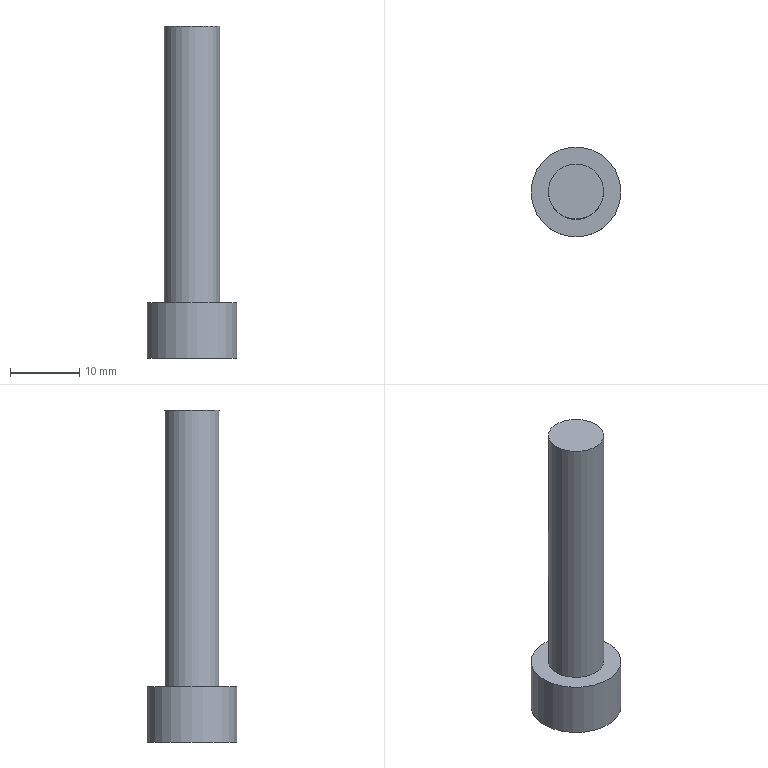Part | STEP file | 1 solid | 12 faces | box 13 x 13 x 48 mm | volume 2908 mm3 | plane 10 | cylinder 2 | commonest cylinder face diameters 8 x1 13 x1
STEP:
#1=CARTESIAN_POINT('',(0.,0.,0.));
#2=DIRECTION('',(0.,0.,1.));
#3=DIRECTION('',(1.,0.,0.));
#4=AXIS2_PLACEMENT_3D('',#1,#2,#3);
#5=CARTESIAN_POINT('',(1889.747,374.48,12.419));
#6=VERTEX_POINT('',#5);
#7=CARTESIAN_POINT('',(1896.247,374.48,12.419));
#8=DIRECTION('',(0.,0.,-1.));
#9=DIRECTION('',(-1.,0.,0.));
#10=AXIS2_PLACEMENT_3D('',#7,#8,#9);
#11=CIRCLE('',#10,6.5);
#12=CARTESIAN_POINT('',(1889.747,374.48,12.419));
#13=DIRECTION('',(0.,0.,1.));
#14=DIRECTION('',(1.,0.,0.));
#15=AXIS2_PLACEMENT_3D('',#12,#13,#14);
#16=PLANE('',#15);
#17=CARTESIAN_POINT('',(0.,0.));
#18=CARTESIAN_POINT('',(0.,11.258));
#19=CARTESIAN_POINT('',(9.75,5.629));
#20=CARTESIAN_POINT('',(19.5,0.));
#21=CARTESIAN_POINT('',(9.75,-5.629));
#22=CARTESIAN_POINT('',(0.,-11.258));
#23=CARTESIAN_POINT('',(0.,0.));
#24=(BOUNDED_CURVE()B_SPLINE_CURVE(2,(#17,#18,#19,#20,#21,#22,#23),.UNSPECIFIED.,.T.,.F.)B_SPLINE_CURVE_WITH_KNOTS((1,2,2,2,2,1),(-2.094,0.,2.094,4.189,6.283,8.378),.UNSPECIFIED.)CURVE()GEOMETRIC_REPRESENTATION_ITEM()RATIONAL_B_SPLINE_CURVE((1.,0.5,1.,0.5,1.,0.5,1.))REPRESENTATION_ITEM(''));
#25=(GEOMETRIC_REPRESENTATION_CONTEXT(2)PARAMETRIC_REPRESENTATION_CONTEXT()REPRESENTATION_CONTEXT('',''));
#26=DEFINITIONAL_REPRESENTATION('',(#24),#25);
#27=PCURVE('',#16,#26);
#28=CARTESIAN_POINT('',(1896.247,374.48,67.319));
#29=DIRECTION('',(0.,0.,-1.));
#30=DIRECTION('',(-1.,0.,0.));
#31=AXIS2_PLACEMENT_3D('',#28,#29,#30);
#32=CYLINDRICAL_SURFACE('',#31,6.5);
#33=CARTESIAN_POINT('',(0.,54.9));
#34=DIRECTION('',(1.,0.));
#35=VECTOR('',#34,1.);
#36=LINE('',#33,#35);
#37=(GEOMETRIC_REPRESENTATION_CONTEXT(2)PARAMETRIC_REPRESENTATION_CONTEXT()REPRESENTATION_CONTEXT('',''));
#38=DEFINITIONAL_REPRESENTATION('',(#36),#37);
#39=PCURVE('',#32,#38);
#40=SURFACE_CURVE('',#11,(#27,#39),.PCURVE_S1.);
#41=EDGE_CURVE('',#6,#6,#40,.T.);
#42=ORIENTED_EDGE('',*,*,#41,.T.);
#43=EDGE_LOOP('',(#42));
#44=FACE_BOUND('',#43,.T.);
#45=CARTESIAN_POINT('',(1897.979,377.48,12.419));
#46=VERTEX_POINT('',#45);
#47=CARTESIAN_POINT('',(1894.515,377.48,12.419));
#48=VERTEX_POINT('',#47);
#49=CARTESIAN_POINT('',(1897.979,377.48,12.419));
#50=DIRECTION('',(-1.,0.,0.));
#51=VECTOR('',#50,1.);
#52=LINE('',#49,#51);
#53=CARTESIAN_POINT('',(8.232,3.));
#54=DIRECTION('',(-1.,0.));
#55=VECTOR('',#54,1.);
#56=LINE('',#53,#55);
#57=(GEOMETRIC_REPRESENTATION_CONTEXT(2)PARAMETRIC_REPRESENTATION_CONTEXT()REPRESENTATION_CONTEXT('',''));
#58=DEFINITIONAL_REPRESENTATION('',(#56),#57);
#59=PCURVE('',#16,#58);
#60=CARTESIAN_POINT('',(1897.979,377.48,17.699));
#61=DIRECTION('',(0.,-1.,0.));
#62=DIRECTION('',(-1.,0.,0.));
#63=AXIS2_PLACEMENT_3D('',#60,#61,#62);
#64=PLANE('',#63);
#65=CARTESIAN_POINT('',(0.,5.28));
#66=DIRECTION('',(1.,0.));
#67=VECTOR('',#66,1.);
#68=LINE('',#65,#67);
#69=(GEOMETRIC_REPRESENTATION_CONTEXT(2)PARAMETRIC_REPRESENTATION_CONTEXT()REPRESENTATION_CONTEXT('',''));
#70=DEFINITIONAL_REPRESENTATION('',(#68),#69);
#71=PCURVE('',#64,#70);
#72=SURFACE_CURVE('',#52,(#59,#71),.PCURVE_S1.);
#73=EDGE_CURVE('',#46,#48,#72,.T.);
#74=ORIENTED_EDGE('',*,*,#73,.T.);
#75=CARTESIAN_POINT('',(1892.783,374.48,12.419));
#76=VERTEX_POINT('',#75);
#77=CARTESIAN_POINT('',(1894.515,377.48,12.419));
#78=DIRECTION('',(-0.5,-0.866,0.));
#79=VECTOR('',#78,1.);
#80=LINE('',#77,#79);
#81=CARTESIAN_POINT('',(4.768,3.));
#82=DIRECTION('',(-0.5,-0.866));
#83=VECTOR('',#82,1.);
#84=LINE('',#81,#83);
#85=(GEOMETRIC_REPRESENTATION_CONTEXT(2)PARAMETRIC_REPRESENTATION_CONTEXT()REPRESENTATION_CONTEXT('',''));
#86=DEFINITIONAL_REPRESENTATION('',(#84),#85);
#87=PCURVE('',#16,#86);
#88=CARTESIAN_POINT('',(1894.515,377.48,17.699));
#89=DIRECTION('',(0.866,-0.5,0.));
#90=DIRECTION('',(-0.5,-0.866,0.));
#91=AXIS2_PLACEMENT_3D('',#88,#89,#90);
#92=PLANE('',#91);
#93=CARTESIAN_POINT('',(0.,5.28));
#94=DIRECTION('',(1.,0.));
#95=VECTOR('',#94,1.);
#96=LINE('',#93,#95);
#97=(GEOMETRIC_REPRESENTATION_CONTEXT(2)PARAMETRIC_REPRESENTATION_CONTEXT()REPRESENTATION_CONTEXT('',''));
#98=DEFINITIONAL_REPRESENTATION('',(#96),#97);
#99=PCURVE('',#92,#98);
#100=SURFACE_CURVE('',#80,(#87,#99),.PCURVE_S1.);
#101=EDGE_CURVE('',#48,#76,#100,.T.);
#102=ORIENTED_EDGE('',*,*,#101,.T.);
#103=CARTESIAN_POINT('',(1894.515,371.48,12.419));
#104=VERTEX_POINT('',#103);
#105=CARTESIAN_POINT('',(1892.783,374.48,12.419));
#106=DIRECTION('',(0.5,-0.866,0.));
#107=VECTOR('',#106,1.);
#108=LINE('',#105,#107);
#109=CARTESIAN_POINT('',(3.036,0.));
#110=DIRECTION('',(0.5,-0.866));
#111=VECTOR('',#110,1.);
#112=LINE('',#109,#111);
#113=(GEOMETRIC_REPRESENTATION_CONTEXT(2)PARAMETRIC_REPRESENTATION_CONTEXT()REPRESENTATION_CONTEXT('',''));
#114=DEFINITIONAL_REPRESENTATION('',(#112),#113);
#115=PCURVE('',#16,#114);
#116=CARTESIAN_POINT('',(1892.783,374.48,17.699));
#117=DIRECTION('',(0.866,0.5,0.));
#118=DIRECTION('',(0.5,-0.866,0.));
#119=AXIS2_PLACEMENT_3D('',#116,#117,#118);
#120=PLANE('',#119);
#121=CARTESIAN_POINT('',(0.,5.28));
#122=DIRECTION('',(1.,0.));
#123=VECTOR('',#122,1.);
#124=LINE('',#121,#123);
#125=(GEOMETRIC_REPRESENTATION_CONTEXT(2)PARAMETRIC_REPRESENTATION_CONTEXT()REPRESENTATION_CONTEXT('',''));
#126=DEFINITIONAL_REPRESENTATION('',(#124),#125);
#127=PCURVE('',#120,#126);
#128=SURFACE_CURVE('',#108,(#115,#127),.PCURVE_S1.);
#129=EDGE_CURVE('',#76,#104,#128,.T.);
#130=ORIENTED_EDGE('',*,*,#129,.T.);
#131=CARTESIAN_POINT('',(1897.979,371.48,12.419));
#132=VERTEX_POINT('',#131);
#133=CARTESIAN_POINT('',(1894.515,371.48,12.419));
#134=DIRECTION('',(1.,0.,0.));
#135=VECTOR('',#134,1.);
#136=LINE('',#133,#135);
#137=CARTESIAN_POINT('',(4.768,-3.));
#138=DIRECTION('',(1.,0.));
#139=VECTOR('',#138,1.);
#140=LINE('',#137,#139);
#141=(GEOMETRIC_REPRESENTATION_CONTEXT(2)PARAMETRIC_REPRESENTATION_CONTEXT()REPRESENTATION_CONTEXT('',''));
#142=DEFINITIONAL_REPRESENTATION('',(#140),#141);
#143=PCURVE('',#16,#142);
#144=CARTESIAN_POINT('',(1894.515,371.48,17.699));
#145=DIRECTION('',(0.,1.,0.));
#146=DIRECTION('',(1.,0.,0.));
#147=AXIS2_PLACEMENT_3D('',#144,#145,#146);
#148=PLANE('',#147);
#149=CARTESIAN_POINT('',(0.,5.28));
#150=DIRECTION('',(1.,0.));
#151=VECTOR('',#150,1.);
#152=LINE('',#149,#151);
#153=(GEOMETRIC_REPRESENTATION_CONTEXT(2)PARAMETRIC_REPRESENTATION_CONTEXT()REPRESENTATION_CONTEXT('',''));
#154=DEFINITIONAL_REPRESENTATION('',(#152),#153);
#155=PCURVE('',#148,#154);
#156=SURFACE_CURVE('',#136,(#143,#155),.PCURVE_S1.);
#157=EDGE_CURVE('',#104,#132,#156,.T.);
#158=ORIENTED_EDGE('',*,*,#157,.T.);
#159=CARTESIAN_POINT('',(1899.711,374.48,12.419));
#160=VERTEX_POINT('',#159);
#161=CARTESIAN_POINT('',(1897.979,371.48,12.419));
#162=DIRECTION('',(0.5,0.866,0.));
#163=VECTOR('',#162,1.);
#164=LINE('',#161,#163);
#165=CARTESIAN_POINT('',(8.232,-3.));
#166=DIRECTION('',(0.5,0.866));
#167=VECTOR('',#166,1.);
#168=LINE('',#165,#167);
#169=(GEOMETRIC_REPRESENTATION_CONTEXT(2)PARAMETRIC_REPRESENTATION_CONTEXT()REPRESENTATION_CONTEXT('',''));
#170=DEFINITIONAL_REPRESENTATION('',(#168),#169);
#171=PCURVE('',#16,#170);
#172=CARTESIAN_POINT('',(1897.979,371.48,17.699));
#173=DIRECTION('',(-0.866,0.5,0.));
#174=DIRECTION('',(0.5,0.866,0.));
#175=AXIS2_PLACEMENT_3D('',#172,#173,#174);
#176=PLANE('',#175);
#177=CARTESIAN_POINT('',(0.,5.28));
#178=DIRECTION('',(1.,0.));
#179=VECTOR('',#178,1.);
#180=LINE('',#177,#179);
#181=(GEOMETRIC_REPRESENTATION_CONTEXT(2)PARAMETRIC_REPRESENTATION_CONTEXT()REPRESENTATION_CONTEXT('',''));
#182=DEFINITIONAL_REPRESENTATION('',(#180),#181);
#183=PCURVE('',#176,#182);
#184=SURFACE_CURVE('',#164,(#171,#183),.PCURVE_S1.);
#185=EDGE_CURVE('',#132,#160,#184,.T.);
#186=ORIENTED_EDGE('',*,*,#185,.T.);
#187=CARTESIAN_POINT('',(1899.711,374.48,12.419));
#188=DIRECTION('',(-0.5,0.866,0.));
#189=VECTOR('',#188,1.);
#190=LINE('',#187,#189);
#191=CARTESIAN_POINT('',(9.964,0.));
#192=DIRECTION('',(-0.5,0.866));
#193=VECTOR('',#192,1.);
#194=LINE('',#191,#193);
#195=(GEOMETRIC_REPRESENTATION_CONTEXT(2)PARAMETRIC_REPRESENTATION_CONTEXT()REPRESENTATION_CONTEXT('',''));
#196=DEFINITIONAL_REPRESENTATION('',(#194),#195);
#197=PCURVE('',#16,#196);
#198=CARTESIAN_POINT('',(1899.711,374.48,17.699));
#199=DIRECTION('',(-0.866,-0.5,0.));
#200=DIRECTION('',(-0.5,0.866,0.));
#201=AXIS2_PLACEMENT_3D('',#198,#199,#200);
#202=PLANE('',#201);
#203=CARTESIAN_POINT('',(0.,5.28));
#204=DIRECTION('',(1.,0.));
#205=VECTOR('',#204,1.);
#206=LINE('',#203,#205);
#207=(GEOMETRIC_REPRESENTATION_CONTEXT(2)PARAMETRIC_REPRESENTATION_CONTEXT()REPRESENTATION_CONTEXT('',''));
#208=DEFINITIONAL_REPRESENTATION('',(#206),#207);
#209=PCURVE('',#202,#208);
#210=SURFACE_CURVE('',#190,(#197,#209),.PCURVE_S1.);
#211=EDGE_CURVE('',#160,#46,#210,.T.);
#212=ORIENTED_EDGE('',*,*,#211,.T.);
#213=EDGE_LOOP('',(#74,#102,#130,#158,#186,#212));
#214=FACE_BOUND('',#213,.T.);
#215=ADVANCED_FACE('',(#44,#214),#16,.F.);
#216=ORIENTED_EDGE('',*,*,#41,.F.);
#217=CARTESIAN_POINT('',(1889.747,374.48,20.419));
#218=VERTEX_POINT('',#217);
#219=CARTESIAN_POINT('',(1889.747,374.48,20.419));
#220=CARTESIAN_POINT('',(1889.747,374.48,12.419));
#221=B_SPLINE_CURVE_WITH_KNOTS('',1,(#219,#220),.UNSPECIFIED.,.F.,.F.,(2,2),(46.9,54.9),.PIECEWISE_BEZIER_KNOTS.);
#222=CARTESIAN_POINT('',(0.,0.));
#223=DIRECTION('',(0.,1.));
#224=VECTOR('',#223,1.);
#225=LINE('',#222,#224);
#226=(GEOMETRIC_REPRESENTATION_CONTEXT(2)PARAMETRIC_REPRESENTATION_CONTEXT()REPRESENTATION_CONTEXT('',''));
#227=DEFINITIONAL_REPRESENTATION('',(#225),#226);
#228=PCURVE('',#32,#227);
#229=CARTESIAN_POINT('',(6.283,0.));
#230=DIRECTION('',(0.,1.));
#231=VECTOR('',#230,1.);
#232=LINE('',#229,#231);
#233=(GEOMETRIC_REPRESENTATION_CONTEXT(2)PARAMETRIC_REPRESENTATION_CONTEXT()REPRESENTATION_CONTEXT('',''));
#234=DEFINITIONAL_REPRESENTATION('',(#232),#233);
#235=PCURVE('',#32,#234);
#236=SEAM_CURVE('',#221,(#228,#235),.PCURVE_S1.);
#237=EDGE_CURVE('',#218,#6,#236,.T.);
#238=ORIENTED_EDGE('',*,*,#237,.F.);
#239=CARTESIAN_POINT('',(1896.247,374.48,20.419));
#240=DIRECTION('',(0.,0.,-1.));
#241=DIRECTION('',(-1.,0.,0.));
#242=AXIS2_PLACEMENT_3D('',#239,#240,#241);
#243=CIRCLE('',#242,6.5);
#244=CARTESIAN_POINT('',(0.,46.9));
#245=DIRECTION('',(1.,0.));
#246=VECTOR('',#245,1.);
#247=LINE('',#244,#246);
#248=(GEOMETRIC_REPRESENTATION_CONTEXT(2)PARAMETRIC_REPRESENTATION_CONTEXT()REPRESENTATION_CONTEXT('',''));
#249=DEFINITIONAL_REPRESENTATION('',(#247),#248);
#250=PCURVE('',#32,#249);
#251=CARTESIAN_POINT('',(1892.247,374.48,20.419));
#252=DIRECTION('',(0.,0.,-1.));
#253=DIRECTION('',(-1.,0.,0.));
#254=AXIS2_PLACEMENT_3D('',#251,#252,#253);
#255=PLANE('',#254);
#256=CARTESIAN_POINT('',(-4.,0.));
#257=DIRECTION('',(1.,0.));
#258=AXIS2_PLACEMENT_2D('',#256,#257);
#259=CIRCLE('',#258,6.5);
#260=(GEOMETRIC_REPRESENTATION_CONTEXT(2)PARAMETRIC_REPRESENTATION_CONTEXT()REPRESENTATION_CONTEXT('',''));
#261=DEFINITIONAL_REPRESENTATION('',(#259),#260);
#262=PCURVE('',#255,#261);
#263=SURFACE_CURVE('',#243,(#250,#262),.PCURVE_S1.);
#264=EDGE_CURVE('',#218,#218,#263,.T.);
#265=ORIENTED_EDGE('',*,*,#264,.T.);
#266=ORIENTED_EDGE('',*,*,#237,.T.);
#267=EDGE_LOOP('',(#216,#238,#265,#266));
#268=FACE_BOUND('',#267,.T.);
#269=ADVANCED_FACE('',(#268),#32,.T.);
#270=ORIENTED_EDGE('',*,*,#264,.F.);
#271=EDGE_LOOP('',(#270));
#272=FACE_BOUND('',#271,.T.);
#273=CARTESIAN_POINT('',(1892.247,374.48,20.419));
#274=VERTEX_POINT('',#273);
#275=CARTESIAN_POINT('',(1896.247,374.48,20.419));
#276=DIRECTION('',(0.,0.,-1.));
#277=DIRECTION('',(-1.,0.,0.));
#278=AXIS2_PLACEMENT_3D('',#275,#276,#277);
#279=CIRCLE('',#278,4.);
#280=CARTESIAN_POINT('',(-4.,0.));
#281=DIRECTION('',(1.,0.));
#282=AXIS2_PLACEMENT_2D('',#280,#281);
#283=CIRCLE('',#282,4.);
#284=(GEOMETRIC_REPRESENTATION_CONTEXT(2)PARAMETRIC_REPRESENTATION_CONTEXT()REPRESENTATION_CONTEXT('',''));
#285=DEFINITIONAL_REPRESENTATION('',(#283),#284);
#286=PCURVE('',#255,#285);
#287=CARTESIAN_POINT('',(1896.247,374.48,67.319));
#288=DIRECTION('',(0.,0.,-1.));
#289=DIRECTION('',(-1.,0.,0.));
#290=AXIS2_PLACEMENT_3D('',#287,#288,#289);
#291=CYLINDRICAL_SURFACE('',#290,4.);
#292=CARTESIAN_POINT('',(0.,46.9));
#293=DIRECTION('',(1.,0.));
#294=VECTOR('',#293,1.);
#295=LINE('',#292,#294);
#296=(GEOMETRIC_REPRESENTATION_CONTEXT(2)PARAMETRIC_REPRESENTATION_CONTEXT()REPRESENTATION_CONTEXT('',''));
#297=DEFINITIONAL_REPRESENTATION('',(#295),#296);
#298=PCURVE('',#291,#297);
#299=SURFACE_CURVE('',#279,(#286,#298),.PCURVE_S1.);
#300=EDGE_CURVE('',#274,#274,#299,.T.);
#301=ORIENTED_EDGE('',*,*,#300,.T.);
#302=EDGE_LOOP('',(#301));
#303=FACE_BOUND('',#302,.T.);
#304=ADVANCED_FACE('',(#272,#303),#255,.F.);
#305=ORIENTED_EDGE('',*,*,#300,.F.);
#306=CARTESIAN_POINT('',(1892.247,374.48,60.419));
#307=VERTEX_POINT('',#306);
#308=CARTESIAN_POINT('',(1892.247,374.48,60.419));
#309=CARTESIAN_POINT('',(1892.247,374.48,20.419));
#310=B_SPLINE_CURVE_WITH_KNOTS('',1,(#308,#309),.UNSPECIFIED.,.F.,.F.,(2,2),(6.9,46.9),.PIECEWISE_BEZIER_KNOTS.);
#311=CARTESIAN_POINT('',(0.,0.));
#312=DIRECTION('',(0.,1.));
#313=VECTOR('',#312,1.);
#314=LINE('',#311,#313);
#315=(GEOMETRIC_REPRESENTATION_CONTEXT(2)PARAMETRIC_REPRESENTATION_CONTEXT()REPRESENTATION_CONTEXT('',''));
#316=DEFINITIONAL_REPRESENTATION('',(#314),#315);
#317=PCURVE('',#291,#316);
#318=CARTESIAN_POINT('',(6.283,0.));
#319=DIRECTION('',(0.,1.));
#320=VECTOR('',#319,1.);
#321=LINE('',#318,#320);
#322=(GEOMETRIC_REPRESENTATION_CONTEXT(2)PARAMETRIC_REPRESENTATION_CONTEXT()REPRESENTATION_CONTEXT('',''));
#323=DEFINITIONAL_REPRESENTATION('',(#321),#322);
#324=PCURVE('',#291,#323);
#325=SEAM_CURVE('',#310,(#317,#324),.PCURVE_S1.);
#326=EDGE_CURVE('',#307,#274,#325,.T.);
#327=ORIENTED_EDGE('',*,*,#326,.F.);
#328=CARTESIAN_POINT('',(1896.247,374.48,60.419));
#329=DIRECTION('',(0.,0.,-1.));
#330=DIRECTION('',(-1.,0.,0.));
#331=AXIS2_PLACEMENT_3D('',#328,#329,#330);
#332=CIRCLE('',#331,4.);
#333=CARTESIAN_POINT('',(0.,6.9));
#334=DIRECTION('',(1.,0.));
#335=VECTOR('',#334,1.);
#336=LINE('',#333,#335);
#337=(GEOMETRIC_REPRESENTATION_CONTEXT(2)PARAMETRIC_REPRESENTATION_CONTEXT()REPRESENTATION_CONTEXT('',''));
#338=DEFINITIONAL_REPRESENTATION('',(#336),#337);
#339=PCURVE('',#291,#338);
#340=CARTESIAN_POINT('',(1896.247,374.48,60.419));
#341=DIRECTION('',(0.,0.,-1.));
#342=DIRECTION('',(-1.,0.,0.));
#343=AXIS2_PLACEMENT_3D('',#340,#341,#342);
#344=PLANE('',#343);
#345=CARTESIAN_POINT('',(0.,0.));
#346=DIRECTION('',(1.,0.));
#347=AXIS2_PLACEMENT_2D('',#345,#346);
#348=CIRCLE('',#347,4.);
#349=(GEOMETRIC_REPRESENTATION_CONTEXT(2)PARAMETRIC_REPRESENTATION_CONTEXT()REPRESENTATION_CONTEXT('',''));
#350=DEFINITIONAL_REPRESENTATION('',(#348),#349);
#351=PCURVE('',#344,#350);
#352=SURFACE_CURVE('',#332,(#339,#351),.PCURVE_S1.);
#353=EDGE_CURVE('',#307,#307,#352,.T.);
#354=ORIENTED_EDGE('',*,*,#353,.T.);
#355=ORIENTED_EDGE('',*,*,#326,.T.);
#356=EDGE_LOOP('',(#305,#327,#354,#355));
#357=FACE_BOUND('',#356,.T.);
#358=ADVANCED_FACE('',(#357),#291,.T.);
#359=ORIENTED_EDGE('',*,*,#353,.F.);
#360=EDGE_LOOP('',(#359));
#361=FACE_BOUND('',#360,.T.);
#362=ADVANCED_FACE('',(#361),#344,.F.);
#363=ORIENTED_EDGE('',*,*,#73,.F.);
#364=CARTESIAN_POINT('',(1897.979,377.48,17.699));
#365=VERTEX_POINT('',#364);
#366=CARTESIAN_POINT('',(1897.979,377.48,17.699));
#367=DIRECTION('',(0.,0.,1.));
#368=VECTOR('',#367,1.);
#369=LINE('',#366,#368);
#370=CARTESIAN_POINT('',(0.,0.));
#371=DIRECTION('',(0.,-1.));
#372=VECTOR('',#371,1.);
#373=LINE('',#370,#372);
#374=(GEOMETRIC_REPRESENTATION_CONTEXT(2)PARAMETRIC_REPRESENTATION_CONTEXT()REPRESENTATION_CONTEXT('',''));
#375=DEFINITIONAL_REPRESENTATION('',(#373),#374);
#376=PCURVE('',#64,#375);
#377=CARTESIAN_POINT('',(3.464,0.));
#378=DIRECTION('',(0.,-1.));
#379=VECTOR('',#378,1.);
#380=LINE('',#377,#379);
#381=(GEOMETRIC_REPRESENTATION_CONTEXT(2)PARAMETRIC_REPRESENTATION_CONTEXT()REPRESENTATION_CONTEXT('',''));
#382=DEFINITIONAL_REPRESENTATION('',(#380),#381);
#383=PCURVE('',#202,#382);
#384=SURFACE_CURVE('',#369,(#376,#383),.PCURVE_S1.);
#385=EDGE_CURVE('',#46,#365,#384,.T.);
#386=ORIENTED_EDGE('',*,*,#385,.T.);
#387=CARTESIAN_POINT('',(1894.515,377.48,17.699));
#388=VERTEX_POINT('',#387);
#389=CARTESIAN_POINT('',(1897.979,377.48,17.699));
#390=DIRECTION('',(1.,0.,0.));
#391=VECTOR('',#390,1.);
#392=LINE('',#389,#391);
#393=CARTESIAN_POINT('',(0.,0.));
#394=DIRECTION('',(-1.,0.));
#395=VECTOR('',#394,1.);
#396=LINE('',#393,#395);
#397=(GEOMETRIC_REPRESENTATION_CONTEXT(2)PARAMETRIC_REPRESENTATION_CONTEXT()REPRESENTATION_CONTEXT('',''));
#398=DEFINITIONAL_REPRESENTATION('',(#396),#397);
#399=PCURVE('',#64,#398);
#400=CARTESIAN_POINT('',(1896.247,374.48,17.699));
#401=DIRECTION('',(0.,0.,1.));
#402=DIRECTION('',(1.,0.,0.));
#403=AXIS2_PLACEMENT_3D('',#400,#401,#402);
#404=PLANE('',#403);
#405=CARTESIAN_POINT('',(1.732,3.));
#406=DIRECTION('',(1.,0.));
#407=VECTOR('',#406,1.);
#408=LINE('',#405,#407);
#409=(GEOMETRIC_REPRESENTATION_CONTEXT(2)PARAMETRIC_REPRESENTATION_CONTEXT()REPRESENTATION_CONTEXT('',''));
#410=DEFINITIONAL_REPRESENTATION('',(#408),#409);
#411=PCURVE('',#404,#410);
#412=SURFACE_CURVE('',#392,(#399,#411),.PCURVE_S1.);
#413=EDGE_CURVE('',#388,#365,#412,.T.);
#414=ORIENTED_EDGE('',*,*,#413,.F.);
#415=CARTESIAN_POINT('',(1894.515,377.48,17.699));
#416=DIRECTION('',(0.,0.,1.));
#417=VECTOR('',#416,1.);
#418=LINE('',#415,#417);
#419=CARTESIAN_POINT('',(3.464,0.));
#420=DIRECTION('',(0.,-1.));
#421=VECTOR('',#420,1.);
#422=LINE('',#419,#421);
#423=(GEOMETRIC_REPRESENTATION_CONTEXT(2)PARAMETRIC_REPRESENTATION_CONTEXT()REPRESENTATION_CONTEXT('',''));
#424=DEFINITIONAL_REPRESENTATION('',(#422),#423);
#425=PCURVE('',#64,#424);
#426=CARTESIAN_POINT('',(0.,0.));
#427=DIRECTION('',(0.,-1.));
#428=VECTOR('',#427,1.);
#429=LINE('',#426,#428);
#430=(GEOMETRIC_REPRESENTATION_CONTEXT(2)PARAMETRIC_REPRESENTATION_CONTEXT()REPRESENTATION_CONTEXT('',''));
#431=DEFINITIONAL_REPRESENTATION('',(#429),#430);
#432=PCURVE('',#92,#431);
#433=SURFACE_CURVE('',#418,(#425,#432),.PCURVE_S1.);
#434=EDGE_CURVE('',#48,#388,#433,.T.);
#435=ORIENTED_EDGE('',*,*,#434,.F.);
#436=EDGE_LOOP('',(#363,#386,#414,#435));
#437=FACE_BOUND('',#436,.T.);
#438=ADVANCED_FACE('',(#437),#64,.T.);
#439=ORIENTED_EDGE('',*,*,#101,.F.);
#440=ORIENTED_EDGE('',*,*,#434,.T.);
#441=CARTESIAN_POINT('',(1892.783,374.48,17.699));
#442=VERTEX_POINT('',#441);
#443=CARTESIAN_POINT('',(1894.515,377.48,17.699));
#444=DIRECTION('',(0.5,0.866,0.));
#445=VECTOR('',#444,1.);
#446=LINE('',#443,#445);
#447=CARTESIAN_POINT('',(0.,0.));
#448=DIRECTION('',(-1.,0.));
#449=VECTOR('',#448,1.);
#450=LINE('',#447,#449);
#451=(GEOMETRIC_REPRESENTATION_CONTEXT(2)PARAMETRIC_REPRESENTATION_CONTEXT()REPRESENTATION_CONTEXT('',''));
#452=DEFINITIONAL_REPRESENTATION('',(#450),#451);
#453=PCURVE('',#92,#452);
#454=CARTESIAN_POINT('',(-1.732,3.));
#455=DIRECTION('',(0.5,0.866));
#456=VECTOR('',#455,1.);
#457=LINE('',#454,#456);
#458=(GEOMETRIC_REPRESENTATION_CONTEXT(2)PARAMETRIC_REPRESENTATION_CONTEXT()REPRESENTATION_CONTEXT('',''));
#459=DEFINITIONAL_REPRESENTATION('',(#457),#458);
#460=PCURVE('',#404,#459);
#461=SURFACE_CURVE('',#446,(#453,#460),.PCURVE_S1.);
#462=EDGE_CURVE('',#442,#388,#461,.T.);
#463=ORIENTED_EDGE('',*,*,#462,.F.);
#464=CARTESIAN_POINT('',(1892.783,374.48,17.699));
#465=DIRECTION('',(0.,0.,1.));
#466=VECTOR('',#465,1.);
#467=LINE('',#464,#466);
#468=CARTESIAN_POINT('',(3.464,0.));
#469=DIRECTION('',(0.,-1.));
#470=VECTOR('',#469,1.);
#471=LINE('',#468,#470);
#472=(GEOMETRIC_REPRESENTATION_CONTEXT(2)PARAMETRIC_REPRESENTATION_CONTEXT()REPRESENTATION_CONTEXT('',''));
#473=DEFINITIONAL_REPRESENTATION('',(#471),#472);
#474=PCURVE('',#92,#473);
#475=CARTESIAN_POINT('',(0.,0.));
#476=DIRECTION('',(0.,-1.));
#477=VECTOR('',#476,1.);
#478=LINE('',#475,#477);
#479=(GEOMETRIC_REPRESENTATION_CONTEXT(2)PARAMETRIC_REPRESENTATION_CONTEXT()REPRESENTATION_CONTEXT('',''));
#480=DEFINITIONAL_REPRESENTATION('',(#478),#479);
#481=PCURVE('',#120,#480);
#482=SURFACE_CURVE('',#467,(#474,#481),.PCURVE_S1.);
#483=EDGE_CURVE('',#76,#442,#482,.T.);
#484=ORIENTED_EDGE('',*,*,#483,.F.);
#485=EDGE_LOOP('',(#439,#440,#463,#484));
#486=FACE_BOUND('',#485,.T.);
#487=ADVANCED_FACE('',(#486),#92,.T.);
#488=ORIENTED_EDGE('',*,*,#129,.F.);
#489=ORIENTED_EDGE('',*,*,#483,.T.);
#490=CARTESIAN_POINT('',(1894.515,371.48,17.699));
#491=VERTEX_POINT('',#490);
#492=CARTESIAN_POINT('',(1892.783,374.48,17.699));
#493=DIRECTION('',(-0.5,0.866,0.));
#494=VECTOR('',#493,1.);
#495=LINE('',#492,#494);
#496=CARTESIAN_POINT('',(0.,0.));
#497=DIRECTION('',(-1.,0.));
#498=VECTOR('',#497,1.);
#499=LINE('',#496,#498);
#500=(GEOMETRIC_REPRESENTATION_CONTEXT(2)PARAMETRIC_REPRESENTATION_CONTEXT()REPRESENTATION_CONTEXT('',''));
#501=DEFINITIONAL_REPRESENTATION('',(#499),#500);
#502=PCURVE('',#120,#501);
#503=CARTESIAN_POINT('',(-3.464,0.));
#504=DIRECTION('',(-0.5,0.866));
#505=VECTOR('',#504,1.);
#506=LINE('',#503,#505);
#507=(GEOMETRIC_REPRESENTATION_CONTEXT(2)PARAMETRIC_REPRESENTATION_CONTEXT()REPRESENTATION_CONTEXT('',''));
#508=DEFINITIONAL_REPRESENTATION('',(#506),#507);
#509=PCURVE('',#404,#508);
#510=SURFACE_CURVE('',#495,(#502,#509),.PCURVE_S1.);
#511=EDGE_CURVE('',#491,#442,#510,.T.);
#512=ORIENTED_EDGE('',*,*,#511,.F.);
#513=CARTESIAN_POINT('',(1894.515,371.48,17.699));
#514=DIRECTION('',(0.,0.,1.));
#515=VECTOR('',#514,1.);
#516=LINE('',#513,#515);
#517=CARTESIAN_POINT('',(3.464,0.));
#518=DIRECTION('',(0.,-1.));
#519=VECTOR('',#518,1.);
#520=LINE('',#517,#519);
#521=(GEOMETRIC_REPRESENTATION_CONTEXT(2)PARAMETRIC_REPRESENTATION_CONTEXT()REPRESENTATION_CONTEXT('',''));
#522=DEFINITIONAL_REPRESENTATION('',(#520),#521);
#523=PCURVE('',#120,#522);
#524=CARTESIAN_POINT('',(0.,0.));
#525=DIRECTION('',(0.,-1.));
#526=VECTOR('',#525,1.);
#527=LINE('',#524,#526);
#528=(GEOMETRIC_REPRESENTATION_CONTEXT(2)PARAMETRIC_REPRESENTATION_CONTEXT()REPRESENTATION_CONTEXT('',''));
#529=DEFINITIONAL_REPRESENTATION('',(#527),#528);
#530=PCURVE('',#148,#529);
#531=SURFACE_CURVE('',#516,(#523,#530),.PCURVE_S1.);
#532=EDGE_CURVE('',#104,#491,#531,.T.);
#533=ORIENTED_EDGE('',*,*,#532,.F.);
#534=EDGE_LOOP('',(#488,#489,#512,#533));
#535=FACE_BOUND('',#534,.T.);
#536=ADVANCED_FACE('',(#535),#120,.T.);
#537=ORIENTED_EDGE('',*,*,#157,.F.);
#538=ORIENTED_EDGE('',*,*,#532,.T.);
#539=CARTESIAN_POINT('',(1897.979,371.48,17.699));
#540=VERTEX_POINT('',#539);
#541=CARTESIAN_POINT('',(1894.515,371.48,17.699));
#542=DIRECTION('',(-1.,0.,0.));
#543=VECTOR('',#542,1.);
#544=LINE('',#541,#543);
#545=CARTESIAN_POINT('',(0.,0.));
#546=DIRECTION('',(-1.,0.));
#547=VECTOR('',#546,1.);
#548=LINE('',#545,#547);
#549=(GEOMETRIC_REPRESENTATION_CONTEXT(2)PARAMETRIC_REPRESENTATION_CONTEXT()REPRESENTATION_CONTEXT('',''));
#550=DEFINITIONAL_REPRESENTATION('',(#548),#549);
#551=PCURVE('',#148,#550);
#552=CARTESIAN_POINT('',(-1.732,-3.));
#553=DIRECTION('',(-1.,0.));
#554=VECTOR('',#553,1.);
#555=LINE('',#552,#554);
#556=(GEOMETRIC_REPRESENTATION_CONTEXT(2)PARAMETRIC_REPRESENTATION_CONTEXT()REPRESENTATION_CONTEXT('',''));
#557=DEFINITIONAL_REPRESENTATION('',(#555),#556);
#558=PCURVE('',#404,#557);
#559=SURFACE_CURVE('',#544,(#551,#558),.PCURVE_S1.);
#560=EDGE_CURVE('',#540,#491,#559,.T.);
#561=ORIENTED_EDGE('',*,*,#560,.F.);
#562=CARTESIAN_POINT('',(1897.979,371.48,17.699));
#563=DIRECTION('',(0.,0.,1.));
#564=VECTOR('',#563,1.);
#565=LINE('',#562,#564);
#566=CARTESIAN_POINT('',(3.464,0.));
#567=DIRECTION('',(0.,-1.));
#568=VECTOR('',#567,1.);
#569=LINE('',#566,#568);
#570=(GEOMETRIC_REPRESENTATION_CONTEXT(2)PARAMETRIC_REPRESENTATION_CONTEXT()REPRESENTATION_CONTEXT('',''));
#571=DEFINITIONAL_REPRESENTATION('',(#569),#570);
#572=PCURVE('',#148,#571);
#573=CARTESIAN_POINT('',(0.,0.));
#574=DIRECTION('',(0.,-1.));
#575=VECTOR('',#574,1.);
#576=LINE('',#573,#575);
#577=(GEOMETRIC_REPRESENTATION_CONTEXT(2)PARAMETRIC_REPRESENTATION_CONTEXT()REPRESENTATION_CONTEXT('',''));
#578=DEFINITIONAL_REPRESENTATION('',(#576),#577);
#579=PCURVE('',#176,#578);
#580=SURFACE_CURVE('',#565,(#572,#579),.PCURVE_S1.);
#581=EDGE_CURVE('',#132,#540,#580,.T.);
#582=ORIENTED_EDGE('',*,*,#581,.F.);
#583=EDGE_LOOP('',(#537,#538,#561,#582));
#584=FACE_BOUND('',#583,.T.);
#585=ADVANCED_FACE('',(#584),#148,.T.);
#586=ORIENTED_EDGE('',*,*,#185,.F.);
#587=ORIENTED_EDGE('',*,*,#581,.T.);
#588=CARTESIAN_POINT('',(1899.711,374.48,17.699));
#589=VERTEX_POINT('',#588);
#590=CARTESIAN_POINT('',(1897.979,371.48,17.699));
#591=DIRECTION('',(-0.5,-0.866,0.));
#592=VECTOR('',#591,1.);
#593=LINE('',#590,#592);
#594=CARTESIAN_POINT('',(0.,0.));
#595=DIRECTION('',(-1.,0.));
#596=VECTOR('',#595,1.);
#597=LINE('',#594,#596);
#598=(GEOMETRIC_REPRESENTATION_CONTEXT(2)PARAMETRIC_REPRESENTATION_CONTEXT()REPRESENTATION_CONTEXT('',''));
#599=DEFINITIONAL_REPRESENTATION('',(#597),#598);
#600=PCURVE('',#176,#599);
#601=CARTESIAN_POINT('',(1.732,-3.));
#602=DIRECTION('',(-0.5,-0.866));
#603=VECTOR('',#602,1.);
#604=LINE('',#601,#603);
#605=(GEOMETRIC_REPRESENTATION_CONTEXT(2)PARAMETRIC_REPRESENTATION_CONTEXT()REPRESENTATION_CONTEXT('',''));
#606=DEFINITIONAL_REPRESENTATION('',(#604),#605);
#607=PCURVE('',#404,#606);
#608=SURFACE_CURVE('',#593,(#600,#607),.PCURVE_S1.);
#609=EDGE_CURVE('',#589,#540,#608,.T.);
#610=ORIENTED_EDGE('',*,*,#609,.F.);
#611=CARTESIAN_POINT('',(1899.711,374.48,17.699));
#612=DIRECTION('',(0.,0.,1.));
#613=VECTOR('',#612,1.);
#614=LINE('',#611,#613);
#615=CARTESIAN_POINT('',(3.464,0.));
#616=DIRECTION('',(0.,-1.));
#617=VECTOR('',#616,1.);
#618=LINE('',#615,#617);
#619=(GEOMETRIC_REPRESENTATION_CONTEXT(2)PARAMETRIC_REPRESENTATION_CONTEXT()REPRESENTATION_CONTEXT('',''));
#620=DEFINITIONAL_REPRESENTATION('',(#618),#619);
#621=PCURVE('',#176,#620);
#622=CARTESIAN_POINT('',(0.,0.));
#623=DIRECTION('',(0.,-1.));
#624=VECTOR('',#623,1.);
#625=LINE('',#622,#624);
#626=(GEOMETRIC_REPRESENTATION_CONTEXT(2)PARAMETRIC_REPRESENTATION_CONTEXT()REPRESENTATION_CONTEXT('',''));
#627=DEFINITIONAL_REPRESENTATION('',(#625),#626);
#628=PCURVE('',#202,#627);
#629=SURFACE_CURVE('',#614,(#621,#628),.PCURVE_S1.);
#630=EDGE_CURVE('',#160,#589,#629,.T.);
#631=ORIENTED_EDGE('',*,*,#630,.F.);
#632=EDGE_LOOP('',(#586,#587,#610,#631));
#633=FACE_BOUND('',#632,.T.);
#634=ADVANCED_FACE('',(#633),#176,.T.);
#635=ORIENTED_EDGE('',*,*,#211,.F.);
#636=ORIENTED_EDGE('',*,*,#630,.T.);
#637=CARTESIAN_POINT('',(1899.711,374.48,17.699));
#638=DIRECTION('',(0.5,-0.866,0.));
#639=VECTOR('',#638,1.);
#640=LINE('',#637,#639);
#641=CARTESIAN_POINT('',(0.,0.));
#642=DIRECTION('',(-1.,0.));
#643=VECTOR('',#642,1.);
#644=LINE('',#641,#643);
#645=(GEOMETRIC_REPRESENTATION_CONTEXT(2)PARAMETRIC_REPRESENTATION_CONTEXT()REPRESENTATION_CONTEXT('',''));
#646=DEFINITIONAL_REPRESENTATION('',(#644),#645);
#647=PCURVE('',#202,#646);
#648=CARTESIAN_POINT('',(3.464,0.));
#649=DIRECTION('',(0.5,-0.866));
#650=VECTOR('',#649,1.);
#651=LINE('',#648,#650);
#652=(GEOMETRIC_REPRESENTATION_CONTEXT(2)PARAMETRIC_REPRESENTATION_CONTEXT()REPRESENTATION_CONTEXT('',''));
#653=DEFINITIONAL_REPRESENTATION('',(#651),#652);
#654=PCURVE('',#404,#653);
#655=SURFACE_CURVE('',#640,(#647,#654),.PCURVE_S1.);
#656=EDGE_CURVE('',#365,#589,#655,.T.);
#657=ORIENTED_EDGE('',*,*,#656,.F.);
#658=ORIENTED_EDGE('',*,*,#385,.F.);
#659=EDGE_LOOP('',(#635,#636,#657,#658));
#660=FACE_BOUND('',#659,.T.);
#661=ADVANCED_FACE('',(#660),#202,.T.);
#662=ORIENTED_EDGE('',*,*,#413,.T.);
#663=ORIENTED_EDGE('',*,*,#656,.T.);
#664=ORIENTED_EDGE('',*,*,#609,.T.);
#665=ORIENTED_EDGE('',*,*,#560,.T.);
#666=ORIENTED_EDGE('',*,*,#511,.T.);
#667=ORIENTED_EDGE('',*,*,#462,.T.);
#668=EDGE_LOOP('',(#662,#663,#664,#665,#666,#667));
#669=FACE_BOUND('',#668,.T.);
#670=ADVANCED_FACE('',(#669),#404,.F.);
#671=CLOSED_SHELL('',(#215,#269,#304,#358,#362,#438,#487,#536,#585,#634,#661,#670));
#672=MANIFOLD_SOLID_BREP('',#671);
#673=(LENGTH_UNIT()NAMED_UNIT(*)SI_UNIT(.MILLI.,.METRE.));
#674=UNCERTAINTY_MEASURE_WITH_UNIT(LENGTH_MEASURE(0.000002),#673,'','');
#675=(NAMED_UNIT(*)PLANE_ANGLE_UNIT()SI_UNIT($,.RADIAN.));
#676=(NAMED_UNIT(*)SI_UNIT($,.STERADIAN.)SOLID_ANGLE_UNIT());
#677=(GEOMETRIC_REPRESENTATION_CONTEXT(3)GLOBAL_UNCERTAINTY_ASSIGNED_CONTEXT((#674))GLOBAL_UNIT_ASSIGNED_CONTEXT((#673,#675,#676))REPRESENTATION_CONTEXT('',''));
#678=ADVANCED_BREP_SHAPE_REPRESENTATION('',(#4,#672),#677);